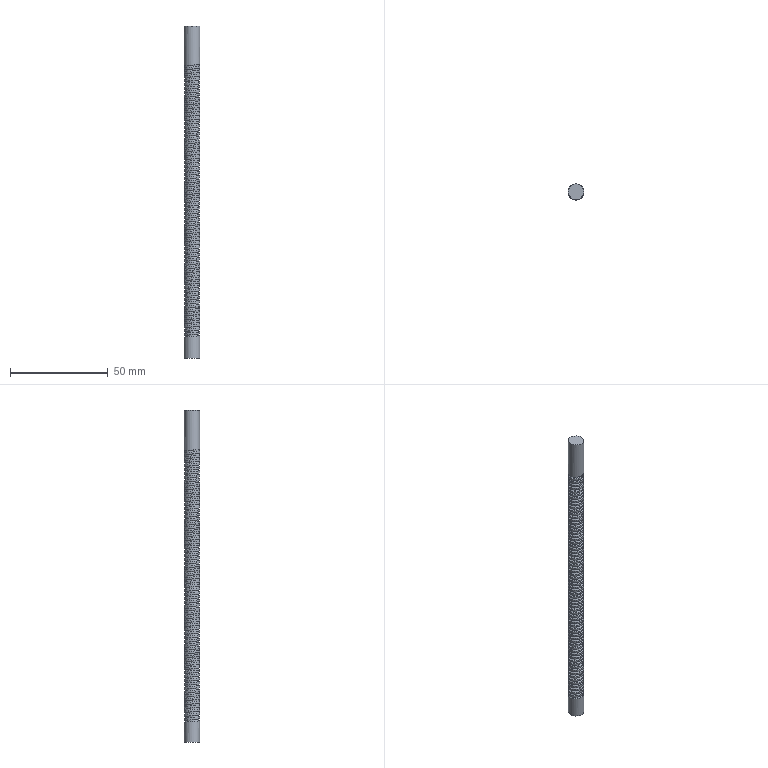Part | NX | features DATUM_CSYS 2, CYLINDER 1, HELIX 1, SKETCH 1, SKIN 1, SUBTRACT 1 | 1 solid | 76 faces | box 8 x 8 x 170 mm | volume 7893 mm3 | cylinder 71 | plane 4 | spline 1 | commonest cylinder face diameters 8 x71